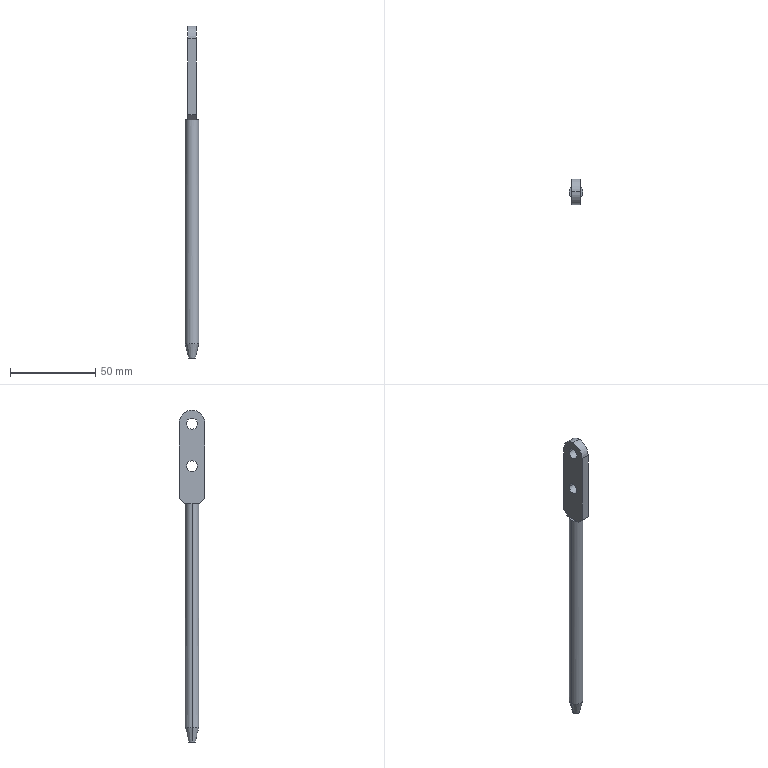Part | SolidWorks | features ICE 2, Chamfer 1, Extrusion 1, Fillet 1, RevCut 1 | 1 solid | 21 faces | box 8 x 15 x 195 mm | volume 10485 mm3 | plane 11 | cylinder 8 | cone 2 | commonest cylinder face diameters 6.5 x4 8 x2 15 x2
STEP:
#1=CARTESIAN_POINT('',(-2.5,-3.25,162.));
#2=VERTEX_POINT('',#1);
#3=CARTESIAN_POINT('',(-2.5,3.25,162.));
#4=VERTEX_POINT('',#3);
#5=CARTESIAN_POINT('',(-2.5,0.,162.));
#6=DIRECTION('',(1.,0.,0.));
#7=DIRECTION('',(0.,1.,0.));
#8=AXIS2_PLACEMENT_3D('',#5,#6,#7);
#9=CIRCLE('',#8,3.25);
#10=EDGE_CURVE('',#2,#4,#9,.T.);
#11=ORIENTED_EDGE('',*,*,#10,.F.);
#12=CARTESIAN_POINT('',(2.5,-3.25,162.));
#13=VERTEX_POINT('',#12);
#14=CARTESIAN_POINT('',(-2.5,-3.25,162.));
#15=DIRECTION('',(1.,0.,0.));
#16=VECTOR('',#15,1000.);
#17=LINE('',#14,#16);
#18=EDGE_CURVE('',#2,#13,#17,.T.);
#19=ORIENTED_EDGE('',*,*,#18,.T.);
#20=CARTESIAN_POINT('',(2.5,3.25,162.));
#21=VERTEX_POINT('',#20);
#22=CARTESIAN_POINT('',(2.5,0.,162.));
#23=DIRECTION('',(1.,0.,0.));
#24=DIRECTION('',(0.,1.,0.));
#25=AXIS2_PLACEMENT_3D('',#22,#23,#24);
#26=CIRCLE('',#25,3.25);
#27=EDGE_CURVE('',#13,#21,#26,.T.);
#28=ORIENTED_EDGE('',*,*,#27,.T.);
#29=CARTESIAN_POINT('',(-2.5,3.25,162.));
#30=DIRECTION('',(1.,0.,0.));
#31=VECTOR('',#30,1000.);
#32=LINE('',#29,#31);
#33=EDGE_CURVE('',#4,#21,#32,.T.);
#34=ORIENTED_EDGE('',*,*,#33,.F.);
#35=EDGE_LOOP('',(#11,#19,#28,#34));
#36=FACE_OUTER_BOUND('',#35,.T.);
#37=CARTESIAN_POINT('',(-2.5,0.,162.));
#38=DIRECTION('',(1.,0.,0.));
#39=DIRECTION('',(0.,1.,0.));
#40=AXIS2_PLACEMENT_3D('',#37,#38,#39);
#41=CYLINDRICAL_SURFACE('',#40,3.25);
#42=ADVANCED_FACE('',(#36),#41,.F.);
#43=CARTESIAN_POINT('',(-2.5,-3.25,187.));
#44=VERTEX_POINT('',#43);
#45=CARTESIAN_POINT('',(-2.5,3.25,187.));
#46=VERTEX_POINT('',#45);
#47=CARTESIAN_POINT('',(-2.5,0.,187.));
#48=DIRECTION('',(1.,0.,0.));
#49=DIRECTION('',(0.,1.,0.));
#50=AXIS2_PLACEMENT_3D('',#47,#48,#49);
#51=CIRCLE('',#50,3.25);
#52=EDGE_CURVE('',#44,#46,#51,.T.);
#53=ORIENTED_EDGE('',*,*,#52,.F.);
#54=CARTESIAN_POINT('',(2.5,-3.25,187.));
#55=VERTEX_POINT('',#54);
#56=CARTESIAN_POINT('',(-2.5,-3.25,187.));
#57=DIRECTION('',(1.,0.,0.));
#58=VECTOR('',#57,1000.);
#59=LINE('',#56,#58);
#60=EDGE_CURVE('',#44,#55,#59,.T.);
#61=ORIENTED_EDGE('',*,*,#60,.T.);
#62=CARTESIAN_POINT('',(2.5,3.25,187.));
#63=VERTEX_POINT('',#62);
#64=CARTESIAN_POINT('',(2.5,0.,187.));
#65=DIRECTION('',(1.,0.,0.));
#66=DIRECTION('',(0.,1.,0.));
#67=AXIS2_PLACEMENT_3D('',#64,#65,#66);
#68=CIRCLE('',#67,3.25);
#69=EDGE_CURVE('',#55,#63,#68,.T.);
#70=ORIENTED_EDGE('',*,*,#69,.T.);
#71=CARTESIAN_POINT('',(-2.5,3.25,187.));
#72=DIRECTION('',(1.,0.,0.));
#73=VECTOR('',#72,1000.);
#74=LINE('',#71,#73);
#75=EDGE_CURVE('',#46,#63,#74,.T.);
#76=ORIENTED_EDGE('',*,*,#75,.F.);
#77=EDGE_LOOP('',(#53,#61,#70,#76));
#78=FACE_OUTER_BOUND('',#77,.T.);
#79=CARTESIAN_POINT('',(-2.5,0.,187.));
#80=DIRECTION('',(1.,0.,0.));
#81=DIRECTION('',(0.,1.,0.));
#82=AXIS2_PLACEMENT_3D('',#79,#80,#81);
#83=CYLINDRICAL_SURFACE('',#82,3.25);
#84=ADVANCED_FACE('',(#78),#83,.F.);
#85=CARTESIAN_POINT('',(1.947,0.,0.));
#86=VERTEX_POINT('',#85);
#87=CARTESIAN_POINT('',(-1.947,0.,0.));
#88=VERTEX_POINT('',#87);
#89=CARTESIAN_POINT('',(0.,0.,0.));
#90=DIRECTION('',(0.,0.,1.));
#91=DIRECTION('',(1.,0.,0.));
#92=AXIS2_PLACEMENT_3D('',#89,#90,#91);
#93=CIRCLE('',#92,1.947);
#94=EDGE_CURVE('',#86,#88,#93,.T.);
#95=ORIENTED_EDGE('',*,*,#94,.T.);
#96=CARTESIAN_POINT('',(-4.,0.,8.412));
#97=VERTEX_POINT('',#96);
#98=CARTESIAN_POINT('',(-4.,0.,8.412));
#99=DIRECTION('',(-0.2371,0.,0.9715));
#100=VECTOR('',#99,1000.);
#101=LINE('',#98,#100);
#102=EDGE_CURVE('',#88,#97,#101,.T.);
#103=ORIENTED_EDGE('',*,*,#102,.T.);
#104=CARTESIAN_POINT('',(4.,0.,8.412));
#105=VERTEX_POINT('',#104);
#106=CARTESIAN_POINT('',(0.,0.,8.412));
#107=DIRECTION('',(0.,0.,1.));
#108=DIRECTION('',(1.,0.,0.));
#109=AXIS2_PLACEMENT_3D('',#106,#107,#108);
#110=CIRCLE('',#109,4.);
#111=EDGE_CURVE('',#105,#97,#110,.T.);
#112=ORIENTED_EDGE('',*,*,#111,.F.);
#113=CARTESIAN_POINT('',(4.,0.,8.412));
#114=DIRECTION('',(0.2371,0.,0.9715));
#115=VECTOR('',#114,1000.);
#116=LINE('',#113,#115);
#117=EDGE_CURVE('',#86,#105,#116,.T.);
#118=ORIENTED_EDGE('',*,*,#117,.F.);
#119=EDGE_LOOP('',(#95,#103,#112,#118));
#120=FACE_OUTER_BOUND('',#119,.T.);
#121=CARTESIAN_POINT('',(0.,0.,8.412));
#122=DIRECTION('',(0.,0.,1.));
#123=DIRECTION('',(1.,0.,0.));
#124=AXIS2_PLACEMENT_3D('',#121,#122,#123);
#125=CONICAL_SURFACE('',#124,4.,0.2394);
#126=ADVANCED_FACE('',(#120),#125,.T.);
#127=CARTESIAN_POINT('',(4.,0.,140.));
#128=VERTEX_POINT('',#127);
#129=CARTESIAN_POINT('',(2.5,3.122,140.));
#130=VERTEX_POINT('',#129);
#131=CARTESIAN_POINT('',(0.,0.,140.));
#132=DIRECTION('',(0.,0.,1.));
#133=DIRECTION('',(1.,0.,0.));
#134=AXIS2_PLACEMENT_3D('',#131,#132,#133);
#135=CIRCLE('',#134,4.);
#136=EDGE_CURVE('',#128,#130,#135,.T.);
#137=ORIENTED_EDGE('',*,*,#136,.F.);
#138=CARTESIAN_POINT('',(4.,0.,140.));
#139=DIRECTION('',(0.,0.,-1.));
#140=VECTOR('',#139,1000.);
#141=LINE('',#138,#140);
#142=EDGE_CURVE('',#128,#105,#141,.T.);
#143=ORIENTED_EDGE('',*,*,#142,.T.);
#144=ORIENTED_EDGE('',*,*,#111,.T.);
#145=CARTESIAN_POINT('',(-4.,0.,140.));
#146=VERTEX_POINT('',#145);
#147=CARTESIAN_POINT('',(-4.,0.,140.));
#148=DIRECTION('',(0.,0.,-1.));
#149=VECTOR('',#148,1000.);
#150=LINE('',#147,#149);
#151=EDGE_CURVE('',#146,#97,#150,.T.);
#152=ORIENTED_EDGE('',*,*,#151,.F.);
#153=CARTESIAN_POINT('',(-2.5,3.122,140.));
#154=VERTEX_POINT('',#153);
#155=CARTESIAN_POINT('',(0.,0.,140.));
#156=DIRECTION('',(0.,0.,1.));
#157=DIRECTION('',(1.,0.,0.));
#158=AXIS2_PLACEMENT_3D('',#155,#156,#157);
#159=CIRCLE('',#158,4.);
#160=EDGE_CURVE('',#154,#146,#159,.T.);
#161=ORIENTED_EDGE('',*,*,#160,.F.);
#162=CARTESIAN_POINT('',(0.,0.,140.));
#163=DIRECTION('',(0.,0.,1.));
#164=DIRECTION('',(1.,0.,0.));
#165=AXIS2_PLACEMENT_3D('',#162,#163,#164);
#166=CIRCLE('',#165,4.);
#167=EDGE_CURVE('',#130,#154,#166,.T.);
#168=ORIENTED_EDGE('',*,*,#167,.F.);
#169=EDGE_LOOP('',(#137,#143,#144,#152,#161,#168));
#170=FACE_OUTER_BOUND('',#169,.T.);
#171=CARTESIAN_POINT('',(0.,0.,140.));
#172=DIRECTION('',(0.,0.,-1.));
#173=DIRECTION('',(-1.,0.,0.));
#174=AXIS2_PLACEMENT_3D('',#171,#172,#173);
#175=CYLINDRICAL_SURFACE('',#174,4.);
#176=ADVANCED_FACE('',(#170),#175,.T.);
#177=CARTESIAN_POINT('',(2.5,-3.122,140.));
#178=VERTEX_POINT('',#177);
#179=CARTESIAN_POINT('',(2.5,7.5,140.));
#180=DIRECTION('',(0.,1.,0.));
#181=VECTOR('',#180,1000.);
#182=LINE('',#179,#181);
#183=EDGE_CURVE('',#178,#130,#182,.T.);
#184=ORIENTED_EDGE('',*,*,#183,.F.);
#185=CARTESIAN_POINT('',(0.,0.,140.));
#186=DIRECTION('',(0.,0.,1.));
#187=DIRECTION('',(1.,0.,0.));
#188=AXIS2_PLACEMENT_3D('',#185,#186,#187);
#189=CIRCLE('',#188,4.);
#190=EDGE_CURVE('',#178,#128,#189,.T.);
#191=ORIENTED_EDGE('',*,*,#190,.T.);
#192=ORIENTED_EDGE('',*,*,#136,.T.);
#193=EDGE_LOOP('',(#184,#191,#192));
#194=FACE_OUTER_BOUND('',#193,.T.);
#195=CARTESIAN_POINT('',(0.,0.,140.));
#196=DIRECTION('',(0.,0.,1.));
#197=DIRECTION('',(1.,0.,0.));
#198=AXIS2_PLACEMENT_3D('',#195,#196,#197);
#199=PLANE('',#198);
#200=ADVANCED_FACE('',(#194),#199,.T.);
#201=ORIENTED_EDGE('',*,*,#142,.F.);
#202=ORIENTED_EDGE('',*,*,#190,.F.);
#203=CARTESIAN_POINT('',(-2.5,-3.122,140.));
#204=VERTEX_POINT('',#203);
#205=CARTESIAN_POINT('',(0.,0.,140.));
#206=DIRECTION('',(0.,0.,1.));
#207=DIRECTION('',(1.,0.,0.));
#208=AXIS2_PLACEMENT_3D('',#205,#206,#207);
#209=CIRCLE('',#208,4.);
#210=EDGE_CURVE('',#204,#178,#209,.T.);
#211=ORIENTED_EDGE('',*,*,#210,.F.);
#212=CARTESIAN_POINT('',(0.,0.,140.));
#213=DIRECTION('',(0.,0.,1.));
#214=DIRECTION('',(1.,0.,0.));
#215=AXIS2_PLACEMENT_3D('',#212,#213,#214);
#216=CIRCLE('',#215,4.);
#217=EDGE_CURVE('',#146,#204,#216,.T.);
#218=ORIENTED_EDGE('',*,*,#217,.F.);
#219=ORIENTED_EDGE('',*,*,#151,.T.);
#220=CARTESIAN_POINT('',(0.,0.,8.412));
#221=DIRECTION('',(0.,0.,1.));
#222=DIRECTION('',(1.,0.,0.));
#223=AXIS2_PLACEMENT_3D('',#220,#221,#222);
#224=CIRCLE('',#223,4.);
#225=EDGE_CURVE('',#97,#105,#224,.T.);
#226=ORIENTED_EDGE('',*,*,#225,.T.);
#227=EDGE_LOOP('',(#201,#202,#211,#218,#219,#226));
#228=FACE_OUTER_BOUND('',#227,.T.);
#229=CARTESIAN_POINT('',(0.,0.,140.));
#230=DIRECTION('',(0.,0.,-1.));
#231=DIRECTION('',(-1.,0.,0.));
#232=AXIS2_PLACEMENT_3D('',#229,#230,#231);
#233=CYLINDRICAL_SURFACE('',#232,4.);
#234=ADVANCED_FACE('',(#228),#233,.T.);
#235=CARTESIAN_POINT('',(-2.5,7.5,140.));
#236=DIRECTION('',(0.,-1.,0.));
#237=VECTOR('',#236,1000.);
#238=LINE('',#235,#237);
#239=EDGE_CURVE('',#154,#204,#238,.T.);
#240=ORIENTED_EDGE('',*,*,#239,.F.);
#241=ORIENTED_EDGE('',*,*,#160,.T.);
#242=ORIENTED_EDGE('',*,*,#217,.T.);
#243=EDGE_LOOP('',(#240,#241,#242));
#244=FACE_OUTER_BOUND('',#243,.T.);
#245=CARTESIAN_POINT('',(0.,0.,140.));
#246=DIRECTION('',(0.,0.,1.));
#247=DIRECTION('',(1.,0.,0.));
#248=AXIS2_PLACEMENT_3D('',#245,#246,#247);
#249=PLANE('',#248);
#250=ADVANCED_FACE('',(#244),#249,.T.);
#251=ORIENTED_EDGE('',*,*,#102,.F.);
#252=CARTESIAN_POINT('',(0.,0.,0.));
#253=DIRECTION('',(0.,0.,1.));
#254=DIRECTION('',(1.,0.,0.));
#255=AXIS2_PLACEMENT_3D('',#252,#253,#254);
#256=CIRCLE('',#255,1.947);
#257=EDGE_CURVE('',#88,#86,#256,.T.);
#258=ORIENTED_EDGE('',*,*,#257,.T.);
#259=ORIENTED_EDGE('',*,*,#117,.T.);
#260=ORIENTED_EDGE('',*,*,#225,.F.);
#261=EDGE_LOOP('',(#251,#258,#259,#260));
#262=FACE_OUTER_BOUND('',#261,.T.);
#263=CARTESIAN_POINT('',(0.,0.,8.412));
#264=DIRECTION('',(0.,0.,1.));
#265=DIRECTION('',(1.,0.,0.));
#266=AXIS2_PLACEMENT_3D('',#263,#264,#265);
#267=CONICAL_SURFACE('',#266,4.,0.2394);
#268=ADVANCED_FACE('',(#262),#267,.T.);
#269=ORIENTED_EDGE('',*,*,#94,.F.);
#270=ORIENTED_EDGE('',*,*,#257,.F.);
#271=EDGE_LOOP('',(#269,#270));
#272=FACE_OUTER_BOUND('',#271,.T.);
#273=CARTESIAN_POINT('',(0.,0.,0.));
#274=DIRECTION('',(0.,0.,1.));
#275=DIRECTION('',(1.,0.,0.));
#276=AXIS2_PLACEMENT_3D('',#273,#274,#275);
#277=PLANE('',#276);
#278=ADVANCED_FACE('',(#272),#277,.F.);
#279=CARTESIAN_POINT('',(-2.5,4.5,140.));
#280=VERTEX_POINT('',#279);
#281=CARTESIAN_POINT('',(-2.5,7.5,140.));
#282=DIRECTION('',(0.,-1.,0.));
#283=VECTOR('',#282,1000.);
#284=LINE('',#281,#283);
#285=EDGE_CURVE('',#280,#154,#284,.T.);
#286=ORIENTED_EDGE('',*,*,#285,.F.);
#287=CARTESIAN_POINT('',(2.5,4.5,140.));
#288=VERTEX_POINT('',#287);
#289=CARTESIAN_POINT('',(2.5,4.5,140.));
#290=DIRECTION('',(1.,0.,0.));
#291=VECTOR('',#290,1000.);
#292=LINE('',#289,#291);
#293=EDGE_CURVE('',#280,#288,#292,.T.);
#294=ORIENTED_EDGE('',*,*,#293,.T.);
#295=CARTESIAN_POINT('',(2.5,7.5,140.));
#296=DIRECTION('',(0.,1.,0.));
#297=VECTOR('',#296,1000.);
#298=LINE('',#295,#297);
#299=EDGE_CURVE('',#130,#288,#298,.T.);
#300=ORIENTED_EDGE('',*,*,#299,.F.);
#301=ORIENTED_EDGE('',*,*,#167,.T.);
#302=EDGE_LOOP('',(#286,#294,#300,#301));
#303=FACE_OUTER_BOUND('',#302,.T.);
#304=CARTESIAN_POINT('',(2.5,-7.5,140.));
#305=DIRECTION('',(0.,0.,1.));
#306=DIRECTION('',(1.,0.,0.));
#307=AXIS2_PLACEMENT_3D('',#304,#305,#306);
#308=PLANE('',#307);
#309=ADVANCED_FACE('',(#303),#308,.F.);
#310=CARTESIAN_POINT('',(2.5,-4.5,140.));
#311=VERTEX_POINT('',#310);
#312=CARTESIAN_POINT('',(2.5,7.5,140.));
#313=DIRECTION('',(0.,1.,0.));
#314=VECTOR('',#313,1000.);
#315=LINE('',#312,#314);
#316=EDGE_CURVE('',#311,#178,#315,.T.);
#317=ORIENTED_EDGE('',*,*,#316,.F.);
#318=CARTESIAN_POINT('',(-2.5,-4.5,140.));
#319=VERTEX_POINT('',#318);
#320=CARTESIAN_POINT('',(2.5,-4.5,140.));
#321=DIRECTION('',(-1.,0.,0.));
#322=VECTOR('',#321,1000.);
#323=LINE('',#320,#322);
#324=EDGE_CURVE('',#311,#319,#323,.T.);
#325=ORIENTED_EDGE('',*,*,#324,.T.);
#326=CARTESIAN_POINT('',(-2.5,7.5,140.));
#327=DIRECTION('',(0.,-1.,0.));
#328=VECTOR('',#327,1000.);
#329=LINE('',#326,#328);
#330=EDGE_CURVE('',#204,#319,#329,.T.);
#331=ORIENTED_EDGE('',*,*,#330,.F.);
#332=ORIENTED_EDGE('',*,*,#210,.T.);
#333=EDGE_LOOP('',(#317,#325,#331,#332));
#334=FACE_OUTER_BOUND('',#333,.T.);
#335=CARTESIAN_POINT('',(2.5,-7.5,140.));
#336=DIRECTION('',(0.,0.,1.));
#337=DIRECTION('',(1.,0.,0.));
#338=AXIS2_PLACEMENT_3D('',#335,#336,#337);
#339=PLANE('',#338);
#340=ADVANCED_FACE('',(#334),#339,.F.);
#341=CARTESIAN_POINT('',(2.5,0.,162.));
#342=DIRECTION('',(1.,0.,0.));
#343=DIRECTION('',(0.,1.,0.));
#344=AXIS2_PLACEMENT_3D('',#341,#342,#343);
#345=CIRCLE('',#344,3.25);
#346=EDGE_CURVE('',#21,#13,#345,.T.);
#347=ORIENTED_EDGE('',*,*,#346,.F.);
#348=ORIENTED_EDGE('',*,*,#27,.F.);
#349=EDGE_LOOP('',(#347,#348));
#350=FACE_BOUND('',#349,.T.);
#351=CARTESIAN_POINT('',(2.5,0.,187.));
#352=DIRECTION('',(1.,0.,0.));
#353=DIRECTION('',(0.,1.,0.));
#354=AXIS2_PLACEMENT_3D('',#351,#352,#353);
#355=CIRCLE('',#354,3.25);
#356=EDGE_CURVE('',#63,#55,#355,.T.);
#357=ORIENTED_EDGE('',*,*,#356,.F.);
#358=ORIENTED_EDGE('',*,*,#69,.F.);
#359=EDGE_LOOP('',(#357,#358));
#360=FACE_BOUND('',#359,.T.);
#361=CARTESIAN_POINT('',(2.5,7.5,187.5));
#362=VERTEX_POINT('',#361);
#363=CARTESIAN_POINT('',(2.5,0.,195.));
#364=VERTEX_POINT('',#363);
#365=CARTESIAN_POINT('',(2.5,0.,187.5));
#366=DIRECTION('',(1.,0.,0.));
#367=DIRECTION('',(0.,-1.,0.));
#368=AXIS2_PLACEMENT_3D('',#365,#366,#367);
#369=CIRCLE('',#368,7.5);
#370=EDGE_CURVE('',#362,#364,#369,.T.);
#371=ORIENTED_EDGE('',*,*,#370,.T.);
#372=CARTESIAN_POINT('',(2.5,-7.5,187.5));
#373=VERTEX_POINT('',#372);
#374=CARTESIAN_POINT('',(2.5,0.,187.5));
#375=DIRECTION('',(1.,0.,0.));
#376=DIRECTION('',(0.,-1.,0.));
#377=AXIS2_PLACEMENT_3D('',#374,#375,#376);
#378=CIRCLE('',#377,7.5);
#379=EDGE_CURVE('',#364,#373,#378,.T.);
#380=ORIENTED_EDGE('',*,*,#379,.T.);
#381=CARTESIAN_POINT('',(2.5,-7.5,143.));
#382=VERTEX_POINT('',#381);
#383=CARTESIAN_POINT('',(2.5,-7.5,195.));
#384=DIRECTION('',(0.,0.,-1.));
#385=VECTOR('',#384,1000.);
#386=LINE('',#383,#385);
#387=EDGE_CURVE('',#373,#382,#386,.T.);
#388=ORIENTED_EDGE('',*,*,#387,.T.);
#389=CARTESIAN_POINT('',(2.5,-7.5,143.));
#390=DIRECTION('',(0.,0.7071,-0.7071));
#391=VECTOR('',#390,1000.);
#392=LINE('',#389,#391);
#393=EDGE_CURVE('',#382,#311,#392,.T.);
#394=ORIENTED_EDGE('',*,*,#393,.T.);
#395=ORIENTED_EDGE('',*,*,#316,.T.);
#396=ORIENTED_EDGE('',*,*,#183,.T.);
#397=ORIENTED_EDGE('',*,*,#299,.T.);
#398=CARTESIAN_POINT('',(2.5,7.5,143.));
#399=VERTEX_POINT('',#398);
#400=CARTESIAN_POINT('',(2.5,7.5,143.));
#401=DIRECTION('',(0.,0.7071,0.7071));
#402=VECTOR('',#401,1000.);
#403=LINE('',#400,#402);
#404=EDGE_CURVE('',#288,#399,#403,.T.);
#405=ORIENTED_EDGE('',*,*,#404,.T.);
#406=CARTESIAN_POINT('',(2.5,7.5,195.));
#407=DIRECTION('',(0.,0.,-1.));
#408=VECTOR('',#407,1000.);
#409=LINE('',#406,#408);
#410=EDGE_CURVE('',#362,#399,#409,.T.);
#411=ORIENTED_EDGE('',*,*,#410,.F.);
#412=EDGE_LOOP('',(#371,#380,#388,#394,#395,#396,#397,#405,#411));
#413=FACE_OUTER_BOUND('',#412,.T.);
#414=CARTESIAN_POINT('',(2.5,7.5,195.));
#415=DIRECTION('',(-1.,0.,0.));
#416=DIRECTION('',(0.,-1.,0.));
#417=AXIS2_PLACEMENT_3D('',#414,#415,#416);
#418=PLANE('',#417);
#419=ADVANCED_FACE('',(#350,#360,#413),#418,.F.);
#420=CARTESIAN_POINT('',(-2.5,7.5,187.5));
#421=VERTEX_POINT('',#420);
#422=CARTESIAN_POINT('',(-2.5,7.5,143.));
#423=VERTEX_POINT('',#422);
#424=CARTESIAN_POINT('',(-2.5,7.5,195.));
#425=DIRECTION('',(0.,0.,-1.));
#426=VECTOR('',#425,1000.);
#427=LINE('',#424,#426);
#428=EDGE_CURVE('',#421,#423,#427,.T.);
#429=ORIENTED_EDGE('',*,*,#428,.F.);
#430=CARTESIAN_POINT('',(2.5,7.5,187.5));
#431=DIRECTION('',(1.,0.,0.));
#432=VECTOR('',#431,1000.);
#433=LINE('',#430,#432);
#434=EDGE_CURVE('',#421,#362,#433,.T.);
#435=ORIENTED_EDGE('',*,*,#434,.T.);
#436=ORIENTED_EDGE('',*,*,#410,.T.);
#437=CARTESIAN_POINT('',(-2.5,7.5,143.));
#438=DIRECTION('',(-1.,0.,0.));
#439=VECTOR('',#438,1000.);
#440=LINE('',#437,#439);
#441=EDGE_CURVE('',#399,#423,#440,.T.);
#442=ORIENTED_EDGE('',*,*,#441,.T.);
#443=EDGE_LOOP('',(#429,#435,#436,#442));
#444=FACE_OUTER_BOUND('',#443,.T.);
#445=CARTESIAN_POINT('',(-2.5,7.5,195.));
#446=DIRECTION('',(0.,-1.,0.));
#447=DIRECTION('',(0.,0.,-1.));
#448=AXIS2_PLACEMENT_3D('',#445,#446,#447);
#449=PLANE('',#448);
#450=ADVANCED_FACE('',(#444),#449,.F.);
#451=CARTESIAN_POINT('',(-2.5,0.,162.));
#452=DIRECTION('',(1.,0.,0.));
#453=DIRECTION('',(0.,1.,0.));
#454=AXIS2_PLACEMENT_3D('',#451,#452,#453);
#455=CIRCLE('',#454,3.25);
#456=EDGE_CURVE('',#4,#2,#455,.T.);
#457=ORIENTED_EDGE('',*,*,#456,.T.);
#458=ORIENTED_EDGE('',*,*,#10,.T.);
#459=EDGE_LOOP('',(#457,#458));
#460=FACE_BOUND('',#459,.T.);
#461=CARTESIAN_POINT('',(-2.5,0.,187.));
#462=DIRECTION('',(1.,0.,0.));
#463=DIRECTION('',(0.,1.,0.));
#464=AXIS2_PLACEMENT_3D('',#461,#462,#463);
#465=CIRCLE('',#464,3.25);
#466=EDGE_CURVE('',#46,#44,#465,.T.);
#467=ORIENTED_EDGE('',*,*,#466,.T.);
#468=ORIENTED_EDGE('',*,*,#52,.T.);
#469=EDGE_LOOP('',(#467,#468));
#470=FACE_BOUND('',#469,.T.);
#471=CARTESIAN_POINT('',(-2.5,-7.5,187.5));
#472=VERTEX_POINT('',#471);
#473=CARTESIAN_POINT('',(-2.5,-7.5,143.));
#474=VERTEX_POINT('',#473);
#475=CARTESIAN_POINT('',(-2.5,-7.5,195.));
#476=DIRECTION('',(0.,0.,-1.));
#477=VECTOR('',#476,1000.);
#478=LINE('',#475,#477);
#479=EDGE_CURVE('',#472,#474,#478,.T.);
#480=ORIENTED_EDGE('',*,*,#479,.F.);
#481=CARTESIAN_POINT('',(-2.5,0.,195.));
#482=VERTEX_POINT('',#481);
#483=CARTESIAN_POINT('',(-2.5,0.,187.5));
#484=DIRECTION('',(-1.,0.,0.));
#485=DIRECTION('',(0.,1.,0.));
#486=AXIS2_PLACEMENT_3D('',#483,#484,#485);
#487=CIRCLE('',#486,7.5);
#488=EDGE_CURVE('',#472,#482,#487,.T.);
#489=ORIENTED_EDGE('',*,*,#488,.T.);
#490=CARTESIAN_POINT('',(-2.5,0.,187.5));
#491=DIRECTION('',(-1.,0.,0.));
#492=DIRECTION('',(0.,1.,0.));
#493=AXIS2_PLACEMENT_3D('',#490,#491,#492);
#494=CIRCLE('',#493,7.5);
#495=EDGE_CURVE('',#482,#421,#494,.T.);
#496=ORIENTED_EDGE('',*,*,#495,.T.);
#497=ORIENTED_EDGE('',*,*,#428,.T.);
#498=CARTESIAN_POINT('',(-2.5,7.5,143.));
#499=DIRECTION('',(0.,-0.7071,-0.7071));
#500=VECTOR('',#499,1000.);
#501=LINE('',#498,#500);
#502=EDGE_CURVE('',#423,#280,#501,.T.);
#503=ORIENTED_EDGE('',*,*,#502,.T.);
#504=ORIENTED_EDGE('',*,*,#285,.T.);
#505=ORIENTED_EDGE('',*,*,#239,.T.);
#506=ORIENTED_EDGE('',*,*,#330,.T.);
#507=CARTESIAN_POINT('',(-2.5,-7.5,143.));
#508=DIRECTION('',(0.,-0.7071,0.7071));
#509=VECTOR('',#508,1000.);
#510=LINE('',#507,#509);
#511=EDGE_CURVE('',#319,#474,#510,.T.);
#512=ORIENTED_EDGE('',*,*,#511,.T.);
#513=EDGE_LOOP('',(#480,#489,#496,#497,#503,#504,#505,#506,#512));
#514=FACE_OUTER_BOUND('',#513,.T.);
#515=CARTESIAN_POINT('',(-2.5,7.5,195.));
#516=DIRECTION('',(1.,0.,0.));
#517=DIRECTION('',(0.,1.,0.));
#518=AXIS2_PLACEMENT_3D('',#515,#516,#517);
#519=PLANE('',#518);
#520=ADVANCED_FACE('',(#460,#470,#514),#519,.F.);
#521=ORIENTED_EDGE('',*,*,#387,.F.);
#522=CARTESIAN_POINT('',(-2.5,-7.5,187.5));
#523=DIRECTION('',(-1.,0.,0.));
#524=VECTOR('',#523,1000.);
#525=LINE('',#522,#524);
#526=EDGE_CURVE('',#373,#472,#525,.T.);
#527=ORIENTED_EDGE('',*,*,#526,.T.);
#528=ORIENTED_EDGE('',*,*,#479,.T.);
#529=CARTESIAN_POINT('',(-2.5,-7.5,143.));
#530=DIRECTION('',(1.,0.,0.));
#531=VECTOR('',#530,1000.);
#532=LINE('',#529,#531);
#533=EDGE_CURVE('',#474,#382,#532,.T.);
#534=ORIENTED_EDGE('',*,*,#533,.T.);
#535=EDGE_LOOP('',(#521,#527,#528,#534));
#536=FACE_OUTER_BOUND('',#535,.T.);
#537=CARTESIAN_POINT('',(-2.5,-7.5,195.));
#538=DIRECTION('',(0.,1.,0.));
#539=DIRECTION('',(0.,0.,1.));
#540=AXIS2_PLACEMENT_3D('',#537,#538,#539);
#541=PLANE('',#540);
#542=ADVANCED_FACE('',(#536),#541,.F.);
#543=ORIENTED_EDGE('',*,*,#511,.F.);
#544=ORIENTED_EDGE('',*,*,#324,.F.);
#545=ORIENTED_EDGE('',*,*,#393,.F.);
#546=ORIENTED_EDGE('',*,*,#533,.F.);
#547=EDGE_LOOP('',(#543,#544,#545,#546));
#548=FACE_OUTER_BOUND('',#547,.T.);
#549=CARTESIAN_POINT('',(-2.5,-7.5,143.));
#550=DIRECTION('',(0.,0.7071,0.7071));
#551=DIRECTION('',(0.,-0.7071,0.7071));
#552=AXIS2_PLACEMENT_3D('',#549,#550,#551);
#553=PLANE('',#552);
#554=ADVANCED_FACE('',(#548),#553,.F.);
#555=ORIENTED_EDGE('',*,*,#404,.F.);
#556=ORIENTED_EDGE('',*,*,#293,.F.);
#557=ORIENTED_EDGE('',*,*,#502,.F.);
#558=ORIENTED_EDGE('',*,*,#441,.F.);
#559=EDGE_LOOP('',(#555,#556,#557,#558));
#560=FACE_OUTER_BOUND('',#559,.T.);
#561=CARTESIAN_POINT('',(-2.5,7.5,143.));
#562=DIRECTION('',(0.,-0.7071,0.7071));
#563=DIRECTION('',(0.,-0.7071,-0.7071));
#564=AXIS2_PLACEMENT_3D('',#561,#562,#563);
#565=PLANE('',#564);
#566=ADVANCED_FACE('',(#560),#565,.F.);
#567=ORIENTED_EDGE('',*,*,#60,.F.);
#568=ORIENTED_EDGE('',*,*,#466,.F.);
#569=ORIENTED_EDGE('',*,*,#75,.T.);
#570=ORIENTED_EDGE('',*,*,#356,.T.);
#571=EDGE_LOOP('',(#567,#568,#569,#570));
#572=FACE_OUTER_BOUND('',#571,.T.);
#573=CARTESIAN_POINT('',(-2.5,0.,187.));
#574=DIRECTION('',(1.,0.,0.));
#575=DIRECTION('',(0.,1.,0.));
#576=AXIS2_PLACEMENT_3D('',#573,#574,#575);
#577=CYLINDRICAL_SURFACE('',#576,3.25);
#578=ADVANCED_FACE('',(#572),#577,.F.);
#579=ORIENTED_EDGE('',*,*,#18,.F.);
#580=ORIENTED_EDGE('',*,*,#456,.F.);
#581=ORIENTED_EDGE('',*,*,#33,.T.);
#582=ORIENTED_EDGE('',*,*,#346,.T.);
#583=EDGE_LOOP('',(#579,#580,#581,#582));
#584=FACE_OUTER_BOUND('',#583,.T.);
#585=CARTESIAN_POINT('',(-2.5,0.,162.));
#586=DIRECTION('',(1.,0.,0.));
#587=DIRECTION('',(0.,1.,0.));
#588=AXIS2_PLACEMENT_3D('',#585,#586,#587);
#589=CYLINDRICAL_SURFACE('',#588,3.25);
#590=ADVANCED_FACE('',(#584),#589,.F.);
#591=ORIENTED_EDGE('',*,*,#434,.F.);
#592=ORIENTED_EDGE('',*,*,#495,.F.);
#593=CARTESIAN_POINT('',(-2.5,0.,195.));
#594=DIRECTION('',(-1.,0.,0.));
#595=VECTOR('',#594,1000.);
#596=LINE('',#593,#595);
#597=EDGE_CURVE('',#364,#482,#596,.T.);
#598=ORIENTED_EDGE('',*,*,#597,.F.);
#599=ORIENTED_EDGE('',*,*,#370,.F.);
#600=EDGE_LOOP('',(#591,#592,#598,#599));
#601=FACE_OUTER_BOUND('',#600,.T.);
#602=CARTESIAN_POINT('',(2.5,0.,187.5));
#603=DIRECTION('',(1.,0.,0.));
#604=DIRECTION('',(0.,0.,-1.));
#605=AXIS2_PLACEMENT_3D('',#602,#603,#604);
#606=CYLINDRICAL_SURFACE('',#605,7.5);
#607=ADVANCED_FACE('',(#601),#606,.T.);
#608=ORIENTED_EDGE('',*,*,#488,.F.);
#609=ORIENTED_EDGE('',*,*,#526,.F.);
#610=ORIENTED_EDGE('',*,*,#379,.F.);
#611=ORIENTED_EDGE('',*,*,#597,.T.);
#612=EDGE_LOOP('',(#608,#609,#610,#611));
#613=FACE_OUTER_BOUND('',#612,.T.);
#614=CARTESIAN_POINT('',(2.5,0.,187.5));
#615=DIRECTION('',(-1.,0.,0.));
#616=DIRECTION('',(0.,0.,1.));
#617=AXIS2_PLACEMENT_3D('',#614,#615,#616);
#618=CYLINDRICAL_SURFACE('',#617,7.5);
#619=ADVANCED_FACE('',(#613),#618,.T.);
#620=CLOSED_SHELL('',(#42,#84,#126,#176,#200,#234,#250,#268,#278,#309,#340,#419,#450,#520,#542,#554,#566,#578,#590,#607,#619));
#621=MANIFOLD_SOLID_BREP('',#620);
#622=CARTESIAN_POINT('',(0.,0.,0.));
#623=DIRECTION('',(0.,0.,1.));
#624=DIRECTION('',(1.,0.,0.));
#625=AXIS2_PLACEMENT_3D('',#622,#623,#624);
#626=(LENGTH_UNIT()NAMED_UNIT(*)SI_UNIT(.MILLI.,.METRE.));
#627=UNCERTAINTY_MEASURE_WITH_UNIT(LENGTH_MEASURE(0.00001),#626,'','');
#628=(NAMED_UNIT(*)PLANE_ANGLE_UNIT()SI_UNIT($,.RADIAN.));
#629=(NAMED_UNIT(*)SI_UNIT($,.STERADIAN.)SOLID_ANGLE_UNIT());
#630=(GEOMETRIC_REPRESENTATION_CONTEXT(3)GLOBAL_UNCERTAINTY_ASSIGNED_CONTEXT((#627))GLOBAL_UNIT_ASSIGNED_CONTEXT((#626,#628,#629))REPRESENTATION_CONTEXT('',''));
#631=ADVANCED_BREP_SHAPE_REPRESENTATION('',(#621,#625),#630);